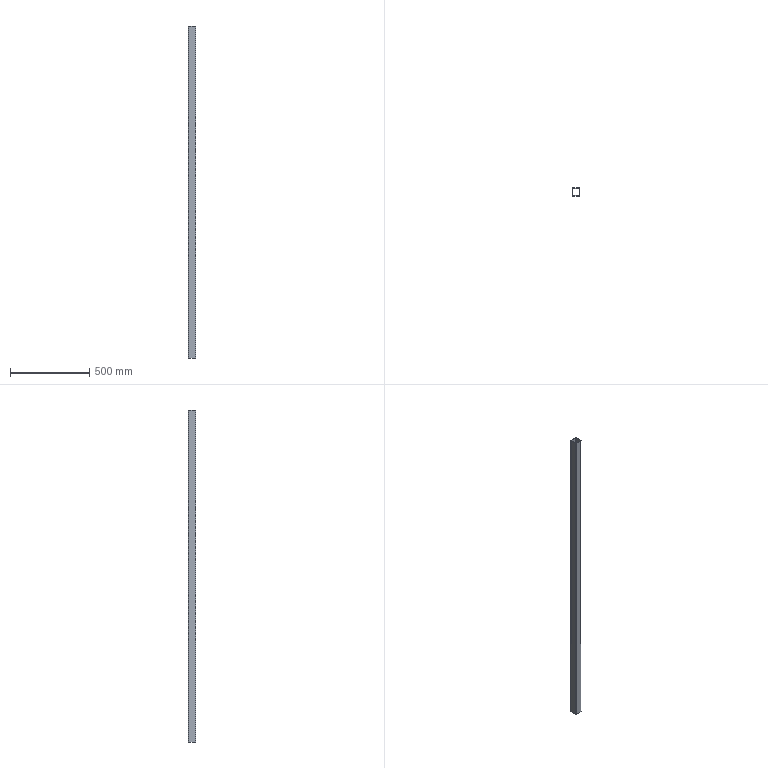Part | SolidWorks | 1 solid | 18 faces | box 50 x 50 x 2100 mm | volume 1135728 mm3 | plane 10 | cylinder 8 | commonest cylinder face diameters 6 x4 12 x4
STEP:
#1=CARTESIAN_POINT('',(19.,25.,1050.));
#2=VERTEX_POINT('',#1);
#3=CARTESIAN_POINT('',(25.,19.,1050.));
#4=VERTEX_POINT('',#3);
#5=CARTESIAN_POINT('',(19.,19.,1050.));
#6=DIRECTION('',(0.,0.,-1.));
#7=DIRECTION('',(-1.,0.,0.));
#8=AXIS2_PLACEMENT_3D('',#5,#6,#7);
#9=CIRCLE('',#8,6.);
#10=EDGE_CURVE('',#2,#4,#9,.T.);
#11=ORIENTED_EDGE('',*,*,#10,.T.);
#12=CARTESIAN_POINT('',(25.,19.,-1050.));
#13=VERTEX_POINT('',#12);
#14=CARTESIAN_POINT('',(25.,19.,-1050.));
#15=DIRECTION('',(0.,0.,1.));
#16=VECTOR('',#15,1000.);
#17=LINE('',#14,#16);
#18=EDGE_CURVE('',#13,#4,#17,.T.);
#19=ORIENTED_EDGE('',*,*,#18,.F.);
#20=CARTESIAN_POINT('',(19.,25.,-1050.));
#21=VERTEX_POINT('',#20);
#22=CARTESIAN_POINT('',(19.,19.,-1050.));
#23=DIRECTION('',(0.,0.,-1.));
#24=DIRECTION('',(-1.,0.,0.));
#25=AXIS2_PLACEMENT_3D('',#22,#23,#24);
#26=CIRCLE('',#25,6.);
#27=EDGE_CURVE('',#21,#13,#26,.T.);
#28=ORIENTED_EDGE('',*,*,#27,.F.);
#29=CARTESIAN_POINT('',(19.,25.,-1050.));
#30=DIRECTION('',(0.,0.,1.));
#31=VECTOR('',#30,1000.);
#32=LINE('',#29,#31);
#33=EDGE_CURVE('',#21,#2,#32,.T.);
#34=ORIENTED_EDGE('',*,*,#33,.T.);
#35=EDGE_LOOP('',(#11,#19,#28,#34));
#36=FACE_OUTER_BOUND('',#35,.T.);
#37=CARTESIAN_POINT('',(19.,19.,-1050.));
#38=DIRECTION('',(0.,0.,1.));
#39=DIRECTION('',(1.,0.,0.));
#40=AXIS2_PLACEMENT_3D('',#37,#38,#39);
#41=CYLINDRICAL_SURFACE('',#40,6.);
#42=ADVANCED_FACE('',(#36),#41,.T.);
#43=CARTESIAN_POINT('',(25.,-19.,1050.));
#44=VERTEX_POINT('',#43);
#45=CARTESIAN_POINT('',(25.,19.,1050.));
#46=DIRECTION('',(0.,-1.,0.));
#47=VECTOR('',#46,1000.);
#48=LINE('',#45,#47);
#49=EDGE_CURVE('',#4,#44,#48,.T.);
#50=ORIENTED_EDGE('',*,*,#49,.T.);
#51=CARTESIAN_POINT('',(25.,-19.,-1050.));
#52=VERTEX_POINT('',#51);
#53=CARTESIAN_POINT('',(25.,-19.,-1050.));
#54=DIRECTION('',(0.,0.,1.));
#55=VECTOR('',#54,1000.);
#56=LINE('',#53,#55);
#57=EDGE_CURVE('',#52,#44,#56,.T.);
#58=ORIENTED_EDGE('',*,*,#57,.F.);
#59=CARTESIAN_POINT('',(25.,19.,-1050.));
#60=DIRECTION('',(0.,-1.,0.));
#61=VECTOR('',#60,1000.);
#62=LINE('',#59,#61);
#63=EDGE_CURVE('',#13,#52,#62,.T.);
#64=ORIENTED_EDGE('',*,*,#63,.F.);
#65=ORIENTED_EDGE('',*,*,#18,.T.);
#66=EDGE_LOOP('',(#50,#58,#64,#65));
#67=FACE_OUTER_BOUND('',#66,.T.);
#68=CARTESIAN_POINT('',(25.,19.,-1050.));
#69=DIRECTION('',(-1.,0.,0.));
#70=DIRECTION('',(0.,0.,1.));
#71=AXIS2_PLACEMENT_3D('',#68,#69,#70);
#72=PLANE('',#71);
#73=ADVANCED_FACE('',(#67),#72,.F.);
#74=CARTESIAN_POINT('',(19.,-25.,1050.));
#75=VERTEX_POINT('',#74);
#76=CARTESIAN_POINT('',(19.,-19.,1050.));
#77=DIRECTION('',(0.,0.,-1.));
#78=DIRECTION('',(-1.,0.,0.));
#79=AXIS2_PLACEMENT_3D('',#76,#77,#78);
#80=CIRCLE('',#79,6.);
#81=EDGE_CURVE('',#44,#75,#80,.T.);
#82=ORIENTED_EDGE('',*,*,#81,.T.);
#83=CARTESIAN_POINT('',(19.,-25.,-1050.));
#84=VERTEX_POINT('',#83);
#85=CARTESIAN_POINT('',(19.,-25.,-1050.));
#86=DIRECTION('',(0.,0.,1.));
#87=VECTOR('',#86,1000.);
#88=LINE('',#85,#87);
#89=EDGE_CURVE('',#84,#75,#88,.T.);
#90=ORIENTED_EDGE('',*,*,#89,.F.);
#91=CARTESIAN_POINT('',(19.,-19.,-1050.));
#92=DIRECTION('',(0.,0.,-1.));
#93=DIRECTION('',(-1.,0.,0.));
#94=AXIS2_PLACEMENT_3D('',#91,#92,#93);
#95=CIRCLE('',#94,6.);
#96=EDGE_CURVE('',#52,#84,#95,.T.);
#97=ORIENTED_EDGE('',*,*,#96,.F.);
#98=ORIENTED_EDGE('',*,*,#57,.T.);
#99=EDGE_LOOP('',(#82,#90,#97,#98));
#100=FACE_OUTER_BOUND('',#99,.T.);
#101=CARTESIAN_POINT('',(19.,-19.,-1050.));
#102=DIRECTION('',(0.,0.,1.));
#103=DIRECTION('',(1.,0.,0.));
#104=AXIS2_PLACEMENT_3D('',#101,#102,#103);
#105=CYLINDRICAL_SURFACE('',#104,6.);
#106=ADVANCED_FACE('',(#100),#105,.T.);
#107=CARTESIAN_POINT('',(-19.,-25.,1050.));
#108=VERTEX_POINT('',#107);
#109=CARTESIAN_POINT('',(-19.,-25.,1050.));
#110=DIRECTION('',(-1.,0.,0.));
#111=VECTOR('',#110,1000.);
#112=LINE('',#109,#111);
#113=EDGE_CURVE('',#75,#108,#112,.T.);
#114=ORIENTED_EDGE('',*,*,#113,.T.);
#115=CARTESIAN_POINT('',(-19.,-25.,-1050.));
#116=VERTEX_POINT('',#115);
#117=CARTESIAN_POINT('',(-19.,-25.,-1050.));
#118=DIRECTION('',(0.,0.,1.));
#119=VECTOR('',#118,1000.);
#120=LINE('',#117,#119);
#121=EDGE_CURVE('',#116,#108,#120,.T.);
#122=ORIENTED_EDGE('',*,*,#121,.F.);
#123=CARTESIAN_POINT('',(-19.,-25.,-1050.));
#124=DIRECTION('',(-1.,0.,0.));
#125=VECTOR('',#124,1000.);
#126=LINE('',#123,#125);
#127=EDGE_CURVE('',#84,#116,#126,.T.);
#128=ORIENTED_EDGE('',*,*,#127,.F.);
#129=ORIENTED_EDGE('',*,*,#89,.T.);
#130=EDGE_LOOP('',(#114,#122,#128,#129));
#131=FACE_OUTER_BOUND('',#130,.T.);
#132=CARTESIAN_POINT('',(-19.,-25.,-1050.));
#133=DIRECTION('',(0.,1.,0.));
#134=DIRECTION('',(0.,0.,1.));
#135=AXIS2_PLACEMENT_3D('',#132,#133,#134);
#136=PLANE('',#135);
#137=ADVANCED_FACE('',(#131),#136,.F.);
#138=CARTESIAN_POINT('',(-25.,-19.,1050.));
#139=VERTEX_POINT('',#138);
#140=CARTESIAN_POINT('',(-19.,-19.,1050.));
#141=DIRECTION('',(0.,0.,-1.));
#142=DIRECTION('',(-1.,0.,0.));
#143=AXIS2_PLACEMENT_3D('',#140,#141,#142);
#144=CIRCLE('',#143,6.);
#145=EDGE_CURVE('',#108,#139,#144,.T.);
#146=ORIENTED_EDGE('',*,*,#145,.T.);
#147=CARTESIAN_POINT('',(-25.,-19.,-1050.));
#148=VERTEX_POINT('',#147);
#149=CARTESIAN_POINT('',(-25.,-19.,-1050.));
#150=DIRECTION('',(0.,0.,1.));
#151=VECTOR('',#150,1000.);
#152=LINE('',#149,#151);
#153=EDGE_CURVE('',#148,#139,#152,.T.);
#154=ORIENTED_EDGE('',*,*,#153,.F.);
#155=CARTESIAN_POINT('',(-19.,-19.,-1050.));
#156=DIRECTION('',(0.,0.,-1.));
#157=DIRECTION('',(-1.,0.,0.));
#158=AXIS2_PLACEMENT_3D('',#155,#156,#157);
#159=CIRCLE('',#158,6.);
#160=EDGE_CURVE('',#116,#148,#159,.T.);
#161=ORIENTED_EDGE('',*,*,#160,.F.);
#162=ORIENTED_EDGE('',*,*,#121,.T.);
#163=EDGE_LOOP('',(#146,#154,#161,#162));
#164=FACE_OUTER_BOUND('',#163,.T.);
#165=CARTESIAN_POINT('',(-19.,-19.,-1050.));
#166=DIRECTION('',(0.,0.,1.));
#167=DIRECTION('',(1.,0.,0.));
#168=AXIS2_PLACEMENT_3D('',#165,#166,#167);
#169=CYLINDRICAL_SURFACE('',#168,6.);
#170=ADVANCED_FACE('',(#164),#169,.T.);
#171=CARTESIAN_POINT('',(-25.,19.,1050.));
#172=VERTEX_POINT('',#171);
#173=CARTESIAN_POINT('',(-25.,-19.,1050.));
#174=DIRECTION('',(0.,1.,0.));
#175=VECTOR('',#174,1000.);
#176=LINE('',#173,#175);
#177=EDGE_CURVE('',#139,#172,#176,.T.);
#178=ORIENTED_EDGE('',*,*,#177,.T.);
#179=CARTESIAN_POINT('',(-25.,19.,-1050.));
#180=VERTEX_POINT('',#179);
#181=CARTESIAN_POINT('',(-25.,19.,-1050.));
#182=DIRECTION('',(0.,0.,1.));
#183=VECTOR('',#182,1000.);
#184=LINE('',#181,#183);
#185=EDGE_CURVE('',#180,#172,#184,.T.);
#186=ORIENTED_EDGE('',*,*,#185,.F.);
#187=CARTESIAN_POINT('',(-25.,-19.,-1050.));
#188=DIRECTION('',(0.,1.,0.));
#189=VECTOR('',#188,1000.);
#190=LINE('',#187,#189);
#191=EDGE_CURVE('',#148,#180,#190,.T.);
#192=ORIENTED_EDGE('',*,*,#191,.F.);
#193=ORIENTED_EDGE('',*,*,#153,.T.);
#194=EDGE_LOOP('',(#178,#186,#192,#193));
#195=FACE_OUTER_BOUND('',#194,.T.);
#196=CARTESIAN_POINT('',(-25.,-19.,-1050.));
#197=DIRECTION('',(1.,0.,0.));
#198=DIRECTION('',(0.,0.,-1.));
#199=AXIS2_PLACEMENT_3D('',#196,#197,#198);
#200=PLANE('',#199);
#201=ADVANCED_FACE('',(#195),#200,.F.);
#202=CARTESIAN_POINT('',(-19.,25.,1050.));
#203=VERTEX_POINT('',#202);
#204=CARTESIAN_POINT('',(-19.,19.,1050.));
#205=DIRECTION('',(0.,0.,-1.));
#206=DIRECTION('',(-1.,0.,0.));
#207=AXIS2_PLACEMENT_3D('',#204,#205,#206);
#208=CIRCLE('',#207,6.);
#209=EDGE_CURVE('',#172,#203,#208,.T.);
#210=ORIENTED_EDGE('',*,*,#209,.T.);
#211=CARTESIAN_POINT('',(-19.,25.,-1050.));
#212=VERTEX_POINT('',#211);
#213=CARTESIAN_POINT('',(-19.,25.,-1050.));
#214=DIRECTION('',(0.,0.,1.));
#215=VECTOR('',#214,1000.);
#216=LINE('',#213,#215);
#217=EDGE_CURVE('',#212,#203,#216,.T.);
#218=ORIENTED_EDGE('',*,*,#217,.F.);
#219=CARTESIAN_POINT('',(-19.,19.,-1050.));
#220=DIRECTION('',(0.,0.,-1.));
#221=DIRECTION('',(-1.,0.,0.));
#222=AXIS2_PLACEMENT_3D('',#219,#220,#221);
#223=CIRCLE('',#222,6.);
#224=EDGE_CURVE('',#180,#212,#223,.T.);
#225=ORIENTED_EDGE('',*,*,#224,.F.);
#226=ORIENTED_EDGE('',*,*,#185,.T.);
#227=EDGE_LOOP('',(#210,#218,#225,#226));
#228=FACE_OUTER_BOUND('',#227,.T.);
#229=CARTESIAN_POINT('',(-19.,19.,-1050.));
#230=DIRECTION('',(0.,0.,1.));
#231=DIRECTION('',(1.,0.,0.));
#232=AXIS2_PLACEMENT_3D('',#229,#230,#231);
#233=CYLINDRICAL_SURFACE('',#232,6.);
#234=ADVANCED_FACE('',(#228),#233,.T.);
#235=CARTESIAN_POINT('',(22.,-19.,1050.));
#236=VERTEX_POINT('',#235);
#237=CARTESIAN_POINT('',(19.,-22.,1050.));
#238=VERTEX_POINT('',#237);
#239=CARTESIAN_POINT('',(19.,-19.,1050.));
#240=DIRECTION('',(0.,0.,-1.));
#241=DIRECTION('',(-1.,0.,0.));
#242=AXIS2_PLACEMENT_3D('',#239,#240,#241);
#243=CIRCLE('',#242,3.);
#244=EDGE_CURVE('',#236,#238,#243,.T.);
#245=ORIENTED_EDGE('',*,*,#244,.F.);
#246=CARTESIAN_POINT('',(22.,-19.,-1050.));
#247=VERTEX_POINT('',#246);
#248=CARTESIAN_POINT('',(22.,-19.,-1050.));
#249=DIRECTION('',(0.,0.,1.));
#250=VECTOR('',#249,1000.);
#251=LINE('',#248,#250);
#252=EDGE_CURVE('',#247,#236,#251,.T.);
#253=ORIENTED_EDGE('',*,*,#252,.F.);
#254=CARTESIAN_POINT('',(19.,-22.,-1050.));
#255=VERTEX_POINT('',#254);
#256=CARTESIAN_POINT('',(19.,-19.,-1050.));
#257=DIRECTION('',(0.,0.,-1.));
#258=DIRECTION('',(-1.,0.,0.));
#259=AXIS2_PLACEMENT_3D('',#256,#257,#258);
#260=CIRCLE('',#259,3.);
#261=EDGE_CURVE('',#247,#255,#260,.T.);
#262=ORIENTED_EDGE('',*,*,#261,.T.);
#263=CARTESIAN_POINT('',(19.,-22.,-1050.));
#264=DIRECTION('',(0.,0.,1.));
#265=VECTOR('',#264,1000.);
#266=LINE('',#263,#265);
#267=EDGE_CURVE('',#255,#238,#266,.T.);
#268=ORIENTED_EDGE('',*,*,#267,.T.);
#269=EDGE_LOOP('',(#245,#253,#262,#268));
#270=FACE_OUTER_BOUND('',#269,.T.);
#271=CARTESIAN_POINT('',(19.,-19.,-1050.));
#272=DIRECTION('',(0.,0.,1.));
#273=DIRECTION('',(1.,0.,0.));
#274=AXIS2_PLACEMENT_3D('',#271,#272,#273);
#275=CYLINDRICAL_SURFACE('',#274,3.);
#276=ADVANCED_FACE('',(#270),#275,.F.);
#277=CARTESIAN_POINT('',(22.,19.,1050.));
#278=VERTEX_POINT('',#277);
#279=CARTESIAN_POINT('',(22.,19.,1050.));
#280=DIRECTION('',(0.,-1.,0.));
#281=VECTOR('',#280,1000.);
#282=LINE('',#279,#281);
#283=EDGE_CURVE('',#278,#236,#282,.T.);
#284=ORIENTED_EDGE('',*,*,#283,.F.);
#285=CARTESIAN_POINT('',(22.,19.,-1050.));
#286=VERTEX_POINT('',#285);
#287=CARTESIAN_POINT('',(22.,19.,-1050.));
#288=DIRECTION('',(0.,0.,1.));
#289=VECTOR('',#288,1000.);
#290=LINE('',#287,#289);
#291=EDGE_CURVE('',#286,#278,#290,.T.);
#292=ORIENTED_EDGE('',*,*,#291,.F.);
#293=CARTESIAN_POINT('',(22.,19.,-1050.));
#294=DIRECTION('',(0.,-1.,0.));
#295=VECTOR('',#294,1000.);
#296=LINE('',#293,#295);
#297=EDGE_CURVE('',#286,#247,#296,.T.);
#298=ORIENTED_EDGE('',*,*,#297,.T.);
#299=ORIENTED_EDGE('',*,*,#252,.T.);
#300=EDGE_LOOP('',(#284,#292,#298,#299));
#301=FACE_OUTER_BOUND('',#300,.T.);
#302=CARTESIAN_POINT('',(22.,19.,-1050.));
#303=DIRECTION('',(-1.,0.,0.));
#304=DIRECTION('',(0.,0.,1.));
#305=AXIS2_PLACEMENT_3D('',#302,#303,#304);
#306=PLANE('',#305);
#307=ADVANCED_FACE('',(#301),#306,.T.);
#308=CARTESIAN_POINT('',(19.,22.,1050.));
#309=VERTEX_POINT('',#308);
#310=CARTESIAN_POINT('',(19.,19.,1050.));
#311=DIRECTION('',(0.,0.,-1.));
#312=DIRECTION('',(-1.,0.,0.));
#313=AXIS2_PLACEMENT_3D('',#310,#311,#312);
#314=CIRCLE('',#313,3.);
#315=EDGE_CURVE('',#309,#278,#314,.T.);
#316=ORIENTED_EDGE('',*,*,#315,.F.);
#317=CARTESIAN_POINT('',(19.,22.,-1050.));
#318=VERTEX_POINT('',#317);
#319=CARTESIAN_POINT('',(19.,22.,-1050.));
#320=DIRECTION('',(0.,0.,1.));
#321=VECTOR('',#320,1000.);
#322=LINE('',#319,#321);
#323=EDGE_CURVE('',#318,#309,#322,.T.);
#324=ORIENTED_EDGE('',*,*,#323,.F.);
#325=CARTESIAN_POINT('',(19.,19.,-1050.));
#326=DIRECTION('',(0.,0.,-1.));
#327=DIRECTION('',(-1.,0.,0.));
#328=AXIS2_PLACEMENT_3D('',#325,#326,#327);
#329=CIRCLE('',#328,3.);
#330=EDGE_CURVE('',#318,#286,#329,.T.);
#331=ORIENTED_EDGE('',*,*,#330,.T.);
#332=ORIENTED_EDGE('',*,*,#291,.T.);
#333=EDGE_LOOP('',(#316,#324,#331,#332));
#334=FACE_OUTER_BOUND('',#333,.T.);
#335=CARTESIAN_POINT('',(19.,19.,-1050.));
#336=DIRECTION('',(0.,0.,1.));
#337=DIRECTION('',(1.,0.,0.));
#338=AXIS2_PLACEMENT_3D('',#335,#336,#337);
#339=CYLINDRICAL_SURFACE('',#338,3.);
#340=ADVANCED_FACE('',(#334),#339,.F.);
#341=CARTESIAN_POINT('',(-19.,22.,1050.));
#342=VERTEX_POINT('',#341);
#343=CARTESIAN_POINT('',(19.,22.,1050.));
#344=DIRECTION('',(1.,0.,0.));
#345=VECTOR('',#344,1000.);
#346=LINE('',#343,#345);
#347=EDGE_CURVE('',#342,#309,#346,.T.);
#348=ORIENTED_EDGE('',*,*,#347,.F.);
#349=CARTESIAN_POINT('',(-19.,22.,-1050.));
#350=VERTEX_POINT('',#349);
#351=CARTESIAN_POINT('',(-19.,22.,-1050.));
#352=DIRECTION('',(0.,0.,1.));
#353=VECTOR('',#352,1000.);
#354=LINE('',#351,#353);
#355=EDGE_CURVE('',#350,#342,#354,.T.);
#356=ORIENTED_EDGE('',*,*,#355,.F.);
#357=CARTESIAN_POINT('',(19.,22.,-1050.));
#358=DIRECTION('',(1.,0.,0.));
#359=VECTOR('',#358,1000.);
#360=LINE('',#357,#359);
#361=EDGE_CURVE('',#350,#318,#360,.T.);
#362=ORIENTED_EDGE('',*,*,#361,.T.);
#363=ORIENTED_EDGE('',*,*,#323,.T.);
#364=EDGE_LOOP('',(#348,#356,#362,#363));
#365=FACE_OUTER_BOUND('',#364,.T.);
#366=CARTESIAN_POINT('',(19.,22.,-1050.));
#367=DIRECTION('',(0.,-1.,0.));
#368=DIRECTION('',(0.,0.,-1.));
#369=AXIS2_PLACEMENT_3D('',#366,#367,#368);
#370=PLANE('',#369);
#371=ADVANCED_FACE('',(#365),#370,.T.);
#372=CARTESIAN_POINT('',(-22.,19.,1050.));
#373=VERTEX_POINT('',#372);
#374=CARTESIAN_POINT('',(-19.,19.,1050.));
#375=DIRECTION('',(0.,0.,-1.));
#376=DIRECTION('',(-1.,0.,0.));
#377=AXIS2_PLACEMENT_3D('',#374,#375,#376);
#378=CIRCLE('',#377,3.);
#379=EDGE_CURVE('',#373,#342,#378,.T.);
#380=ORIENTED_EDGE('',*,*,#379,.F.);
#381=CARTESIAN_POINT('',(-22.,19.,-1050.));
#382=VERTEX_POINT('',#381);
#383=CARTESIAN_POINT('',(-22.,19.,-1050.));
#384=DIRECTION('',(0.,0.,1.));
#385=VECTOR('',#384,1000.);
#386=LINE('',#383,#385);
#387=EDGE_CURVE('',#382,#373,#386,.T.);
#388=ORIENTED_EDGE('',*,*,#387,.F.);
#389=CARTESIAN_POINT('',(-19.,19.,-1050.));
#390=DIRECTION('',(0.,0.,-1.));
#391=DIRECTION('',(-1.,0.,0.));
#392=AXIS2_PLACEMENT_3D('',#389,#390,#391);
#393=CIRCLE('',#392,3.);
#394=EDGE_CURVE('',#382,#350,#393,.T.);
#395=ORIENTED_EDGE('',*,*,#394,.T.);
#396=ORIENTED_EDGE('',*,*,#355,.T.);
#397=EDGE_LOOP('',(#380,#388,#395,#396));
#398=FACE_OUTER_BOUND('',#397,.T.);
#399=CARTESIAN_POINT('',(-19.,19.,-1050.));
#400=DIRECTION('',(0.,0.,1.));
#401=DIRECTION('',(1.,0.,0.));
#402=AXIS2_PLACEMENT_3D('',#399,#400,#401);
#403=CYLINDRICAL_SURFACE('',#402,3.);
#404=ADVANCED_FACE('',(#398),#403,.F.);
#405=CARTESIAN_POINT('',(-22.,-19.,1050.));
#406=VERTEX_POINT('',#405);
#407=CARTESIAN_POINT('',(-22.,-19.,1050.));
#408=DIRECTION('',(0.,1.,0.));
#409=VECTOR('',#408,1000.);
#410=LINE('',#407,#409);
#411=EDGE_CURVE('',#406,#373,#410,.T.);
#412=ORIENTED_EDGE('',*,*,#411,.F.);
#413=CARTESIAN_POINT('',(-22.,-19.,-1050.));
#414=VERTEX_POINT('',#413);
#415=CARTESIAN_POINT('',(-22.,-19.,-1050.));
#416=DIRECTION('',(0.,0.,1.));
#417=VECTOR('',#416,1000.);
#418=LINE('',#415,#417);
#419=EDGE_CURVE('',#414,#406,#418,.T.);
#420=ORIENTED_EDGE('',*,*,#419,.F.);
#421=CARTESIAN_POINT('',(-22.,-19.,-1050.));
#422=DIRECTION('',(0.,1.,0.));
#423=VECTOR('',#422,1000.);
#424=LINE('',#421,#423);
#425=EDGE_CURVE('',#414,#382,#424,.T.);
#426=ORIENTED_EDGE('',*,*,#425,.T.);
#427=ORIENTED_EDGE('',*,*,#387,.T.);
#428=EDGE_LOOP('',(#412,#420,#426,#427));
#429=FACE_OUTER_BOUND('',#428,.T.);
#430=CARTESIAN_POINT('',(-22.,-19.,-1050.));
#431=DIRECTION('',(1.,0.,0.));
#432=DIRECTION('',(0.,0.,-1.));
#433=AXIS2_PLACEMENT_3D('',#430,#431,#432);
#434=PLANE('',#433);
#435=ADVANCED_FACE('',(#429),#434,.T.);
#436=CARTESIAN_POINT('',(-19.,-22.,1050.));
#437=VERTEX_POINT('',#436);
#438=CARTESIAN_POINT('',(-19.,-19.,1050.));
#439=DIRECTION('',(0.,0.,-1.));
#440=DIRECTION('',(-1.,0.,0.));
#441=AXIS2_PLACEMENT_3D('',#438,#439,#440);
#442=CIRCLE('',#441,3.);
#443=EDGE_CURVE('',#437,#406,#442,.T.);
#444=ORIENTED_EDGE('',*,*,#443,.F.);
#445=CARTESIAN_POINT('',(-19.,-22.,-1050.));
#446=VERTEX_POINT('',#445);
#447=CARTESIAN_POINT('',(-19.,-22.,-1050.));
#448=DIRECTION('',(0.,0.,1.));
#449=VECTOR('',#448,1000.);
#450=LINE('',#447,#449);
#451=EDGE_CURVE('',#446,#437,#450,.T.);
#452=ORIENTED_EDGE('',*,*,#451,.F.);
#453=CARTESIAN_POINT('',(-19.,-19.,-1050.));
#454=DIRECTION('',(0.,0.,-1.));
#455=DIRECTION('',(-1.,0.,0.));
#456=AXIS2_PLACEMENT_3D('',#453,#454,#455);
#457=CIRCLE('',#456,3.);
#458=EDGE_CURVE('',#446,#414,#457,.T.);
#459=ORIENTED_EDGE('',*,*,#458,.T.);
#460=ORIENTED_EDGE('',*,*,#419,.T.);
#461=EDGE_LOOP('',(#444,#452,#459,#460));
#462=FACE_OUTER_BOUND('',#461,.T.);
#463=CARTESIAN_POINT('',(-19.,-19.,-1050.));
#464=DIRECTION('',(0.,0.,1.));
#465=DIRECTION('',(1.,0.,0.));
#466=AXIS2_PLACEMENT_3D('',#463,#464,#465);
#467=CYLINDRICAL_SURFACE('',#466,3.);
#468=ADVANCED_FACE('',(#462),#467,.F.);
#469=CARTESIAN_POINT('',(-19.,-22.,1050.));
#470=DIRECTION('',(-1.,0.,0.));
#471=VECTOR('',#470,1000.);
#472=LINE('',#469,#471);
#473=EDGE_CURVE('',#238,#437,#472,.T.);
#474=ORIENTED_EDGE('',*,*,#473,.F.);
#475=ORIENTED_EDGE('',*,*,#267,.F.);
#476=CARTESIAN_POINT('',(-19.,-22.,-1050.));
#477=DIRECTION('',(-1.,0.,0.));
#478=VECTOR('',#477,1000.);
#479=LINE('',#476,#478);
#480=EDGE_CURVE('',#255,#446,#479,.T.);
#481=ORIENTED_EDGE('',*,*,#480,.T.);
#482=ORIENTED_EDGE('',*,*,#451,.T.);
#483=EDGE_LOOP('',(#474,#475,#481,#482));
#484=FACE_OUTER_BOUND('',#483,.T.);
#485=CARTESIAN_POINT('',(-19.,-22.,-1050.));
#486=DIRECTION('',(0.,1.,0.));
#487=DIRECTION('',(0.,0.,1.));
#488=AXIS2_PLACEMENT_3D('',#485,#486,#487);
#489=PLANE('',#488);
#490=ADVANCED_FACE('',(#484),#489,.T.);
#491=CARTESIAN_POINT('',(19.,25.,1050.));
#492=DIRECTION('',(1.,0.,0.));
#493=VECTOR('',#492,1000.);
#494=LINE('',#491,#493);
#495=EDGE_CURVE('',#203,#2,#494,.T.);
#496=ORIENTED_EDGE('',*,*,#495,.T.);
#497=ORIENTED_EDGE('',*,*,#33,.F.);
#498=CARTESIAN_POINT('',(19.,25.,-1050.));
#499=DIRECTION('',(1.,0.,0.));
#500=VECTOR('',#499,1000.);
#501=LINE('',#498,#500);
#502=EDGE_CURVE('',#212,#21,#501,.T.);
#503=ORIENTED_EDGE('',*,*,#502,.F.);
#504=ORIENTED_EDGE('',*,*,#217,.T.);
#505=EDGE_LOOP('',(#496,#497,#503,#504));
#506=FACE_OUTER_BOUND('',#505,.T.);
#507=CARTESIAN_POINT('',(19.,25.,-1050.));
#508=DIRECTION('',(0.,-1.,0.));
#509=DIRECTION('',(0.,0.,-1.));
#510=AXIS2_PLACEMENT_3D('',#507,#508,#509);
#511=PLANE('',#510);
#512=ADVANCED_FACE('',(#506),#511,.F.);
#513=ORIENTED_EDGE('',*,*,#261,.F.);
#514=ORIENTED_EDGE('',*,*,#297,.F.);
#515=ORIENTED_EDGE('',*,*,#330,.F.);
#516=ORIENTED_EDGE('',*,*,#361,.F.);
#517=ORIENTED_EDGE('',*,*,#394,.F.);
#518=ORIENTED_EDGE('',*,*,#425,.F.);
#519=ORIENTED_EDGE('',*,*,#458,.F.);
#520=ORIENTED_EDGE('',*,*,#480,.F.);
#521=EDGE_LOOP('',(#513,#514,#515,#516,#517,#518,#519,#520));
#522=FACE_BOUND('',#521,.T.);
#523=ORIENTED_EDGE('',*,*,#27,.T.);
#524=ORIENTED_EDGE('',*,*,#63,.T.);
#525=ORIENTED_EDGE('',*,*,#96,.T.);
#526=ORIENTED_EDGE('',*,*,#127,.T.);
#527=ORIENTED_EDGE('',*,*,#160,.T.);
#528=ORIENTED_EDGE('',*,*,#191,.T.);
#529=ORIENTED_EDGE('',*,*,#224,.T.);
#530=ORIENTED_EDGE('',*,*,#502,.T.);
#531=EDGE_LOOP('',(#523,#524,#525,#526,#527,#528,#529,#530));
#532=FACE_OUTER_BOUND('',#531,.T.);
#533=CARTESIAN_POINT('',(19.,19.,-1050.));
#534=DIRECTION('',(0.,0.,-1.));
#535=DIRECTION('',(-1.,0.,0.));
#536=AXIS2_PLACEMENT_3D('',#533,#534,#535);
#537=PLANE('',#536);
#538=ADVANCED_FACE('',(#522,#532),#537,.T.);
#539=ORIENTED_EDGE('',*,*,#244,.T.);
#540=ORIENTED_EDGE('',*,*,#473,.T.);
#541=ORIENTED_EDGE('',*,*,#443,.T.);
#542=ORIENTED_EDGE('',*,*,#411,.T.);
#543=ORIENTED_EDGE('',*,*,#379,.T.);
#544=ORIENTED_EDGE('',*,*,#347,.T.);
#545=ORIENTED_EDGE('',*,*,#315,.T.);
#546=ORIENTED_EDGE('',*,*,#283,.T.);
#547=EDGE_LOOP('',(#539,#540,#541,#542,#543,#544,#545,#546));
#548=FACE_BOUND('',#547,.T.);
#549=ORIENTED_EDGE('',*,*,#10,.F.);
#550=ORIENTED_EDGE('',*,*,#495,.F.);
#551=ORIENTED_EDGE('',*,*,#209,.F.);
#552=ORIENTED_EDGE('',*,*,#177,.F.);
#553=ORIENTED_EDGE('',*,*,#145,.F.);
#554=ORIENTED_EDGE('',*,*,#113,.F.);
#555=ORIENTED_EDGE('',*,*,#81,.F.);
#556=ORIENTED_EDGE('',*,*,#49,.F.);
#557=EDGE_LOOP('',(#549,#550,#551,#552,#553,#554,#555,#556));
#558=FACE_OUTER_BOUND('',#557,.T.);
#559=CARTESIAN_POINT('',(19.,19.,1050.));
#560=DIRECTION('',(0.,0.,-1.));
#561=DIRECTION('',(-1.,0.,0.));
#562=AXIS2_PLACEMENT_3D('',#559,#560,#561);
#563=PLANE('',#562);
#564=ADVANCED_FACE('',(#548,#558),#563,.F.);
#565=CLOSED_SHELL('',(#42,#73,#106,#137,#170,#201,#234,#276,#307,#340,#371,#404,#435,#468,#490,#512,#538,#564));
#566=MANIFOLD_SOLID_BREP('',#565);
#567=CARTESIAN_POINT('',(0.,0.,0.));
#568=DIRECTION('',(0.,0.,1.));
#569=DIRECTION('',(1.,0.,0.));
#570=AXIS2_PLACEMENT_3D('',#567,#568,#569);
#571=(LENGTH_UNIT()NAMED_UNIT(*)SI_UNIT(.MILLI.,.METRE.));
#572=UNCERTAINTY_MEASURE_WITH_UNIT(LENGTH_MEASURE(0.00001),#571,'','');
#573=(NAMED_UNIT(*)PLANE_ANGLE_UNIT()SI_UNIT($,.RADIAN.));
#574=(NAMED_UNIT(*)SI_UNIT($,.STERADIAN.)SOLID_ANGLE_UNIT());
#575=(GEOMETRIC_REPRESENTATION_CONTEXT(3)GLOBAL_UNCERTAINTY_ASSIGNED_CONTEXT((#572))GLOBAL_UNIT_ASSIGNED_CONTEXT((#571,#573,#574))REPRESENTATION_CONTEXT('',''));
#576=ADVANCED_BREP_SHAPE_REPRESENTATION('',(#566,#570),#575);